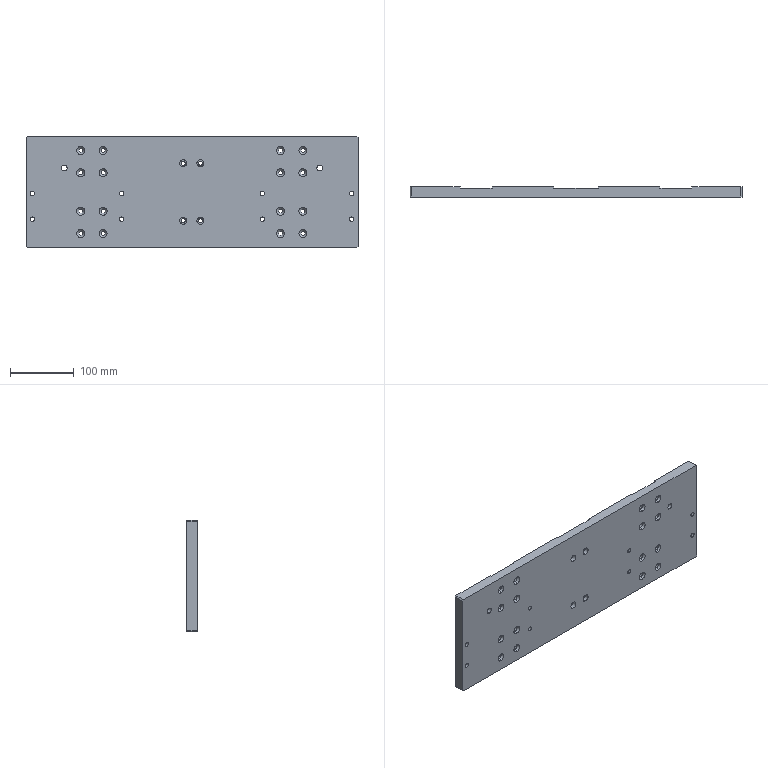Part | STEP file | 1 solid | 126 faces | box 520 x 16 x 175 mm | volume 1376606 mm3 | cylinder 68 | cone 32 | plane 26 | commonest cylinder face diameters 6.6 x40 6.8 x16 11 x8 9 x4